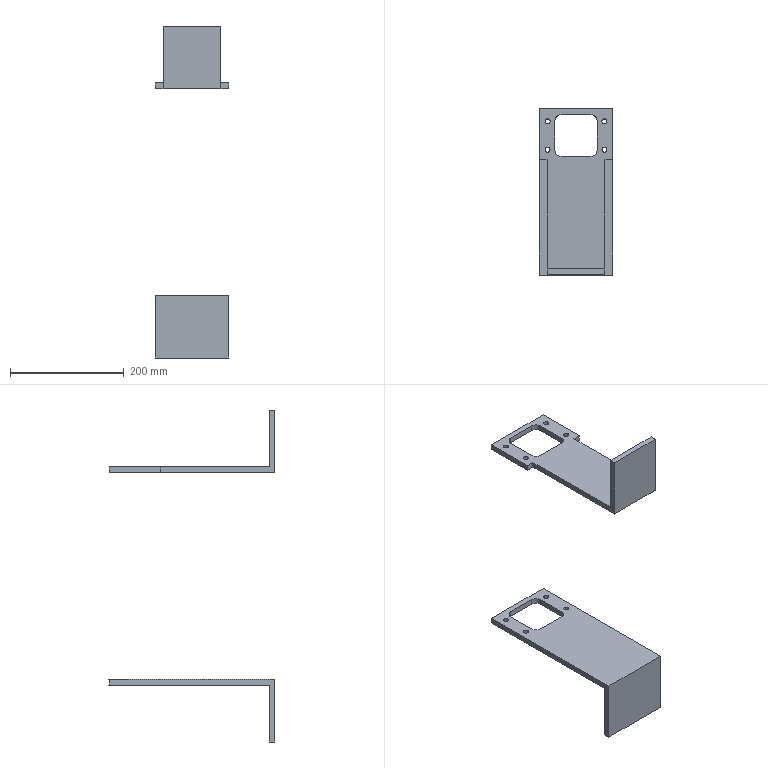Part | NX | 2 solids | 44 faces | box 129 x 292 x 584 mm | volume 817102 mm3 | plane 28 | cylinder 16 | commonest cylinder face diameters 9 x8 21.378 x8
STEP:
#1=CARTESIAN_POINT('',(4645.75,76.144,-128.));
#2=VERTEX_POINT('',#1);
#3=CARTESIAN_POINT('',(4659.262,76.144,-128.));
#4=VERTEX_POINT('',#3);
#5=CARTESIAN_POINT('',(4098.348,76.144,-128.));
#6=DIRECTION('',(1.,0.,0.));
#7=VECTOR('',#6,1.);
#8=LINE('',#5,#7);
#9=EDGE_CURVE('',#2,#4,#8,.T.);
#10=ORIENTED_EDGE('',*,*,#9,.F.);
#11=CARTESIAN_POINT('',(4645.75,76.144,-138.));
#12=VERTEX_POINT('',#11);
#13=CARTESIAN_POINT('',(4645.75,76.144,-128.));
#14=DIRECTION('',(0.,0.,1.));
#15=VECTOR('',#14,1.);
#16=LINE('',#13,#15);
#17=EDGE_CURVE('',#12,#2,#16,.T.);
#18=ORIENTED_EDGE('',*,*,#17,.F.);
#19=CARTESIAN_POINT('',(4659.262,76.144,-138.));
#20=VERTEX_POINT('',#19);
#21=CARTESIAN_POINT('',(4098.348,76.144,-138.));
#22=DIRECTION('',(-1.,0.,0.));
#23=VECTOR('',#22,1.);
#24=LINE('',#21,#23);
#25=EDGE_CURVE('',#20,#12,#24,.T.);
#26=ORIENTED_EDGE('',*,*,#25,.F.);
#27=CARTESIAN_POINT('',(4659.262,76.144,-150.));
#28=DIRECTION('',(0.,0.,1.));
#29=VECTOR('',#28,1.);
#30=LINE('',#27,#29);
#31=EDGE_CURVE('',#20,#4,#30,.T.);
#32=ORIENTED_EDGE('',*,*,#31,.T.);
#33=EDGE_LOOP('',(#10,#18,#26,#32));
#34=FACE_OUTER_BOUND('',#33,.T.);
#35=CARTESIAN_POINT('',(9954.033,76.144,0.));
#36=DIRECTION('',(0.,1.,0.));
#37=DIRECTION('',(0.,0.,1.));
#38=AXIS2_PLACEMENT_3D('',#35,#36,#37);
#39=PLANE('',#38);
#40=ADVANCED_FACE('',(#34),#39,.F.);
#41=CARTESIAN_POINT('',(4659.262,-125.856,-138.));
#42=VERTEX_POINT('',#41);
#43=CARTESIAN_POINT('',(4659.262,-499.191,-138.));
#44=DIRECTION('',(0.,1.,0.));
#45=VECTOR('',#44,1.);
#46=LINE('',#43,#45);
#47=EDGE_CURVE('',#42,#20,#46,.T.);
#48=ORIENTED_EDGE('',*,*,#47,.F.);
#49=CARTESIAN_POINT('',(4659.262,-125.856,-28.));
#50=VERTEX_POINT('',#49);
#51=CARTESIAN_POINT('',(4659.262,-125.856,-150.));
#52=DIRECTION('',(0.,0.,-1.));
#53=VECTOR('',#52,1.);
#54=LINE('',#51,#53);
#55=EDGE_CURVE('',#50,#42,#54,.T.);
#56=ORIENTED_EDGE('',*,*,#55,.F.);
#57=CARTESIAN_POINT('',(4659.262,-115.856,-28.));
#58=VERTEX_POINT('',#57);
#59=CARTESIAN_POINT('',(4659.262,-125.856,-28.));
#60=DIRECTION('',(0.,-1.,0.));
#61=VECTOR('',#60,1.);
#62=LINE('',#59,#61);
#63=EDGE_CURVE('',#58,#50,#62,.T.);
#64=ORIENTED_EDGE('',*,*,#63,.F.);
#65=CARTESIAN_POINT('',(4659.262,-115.856,-128.));
#66=VERTEX_POINT('',#65);
#67=CARTESIAN_POINT('',(4659.262,-115.856,-128.));
#68=DIRECTION('',(0.,0.,1.));
#69=VECTOR('',#68,1.);
#70=LINE('',#67,#69);
#71=EDGE_CURVE('',#66,#58,#70,.T.);
#72=ORIENTED_EDGE('',*,*,#71,.F.);
#73=CARTESIAN_POINT('',(4659.262,-499.191,-128.));
#74=DIRECTION('',(0.,-1.,0.));
#75=VECTOR('',#74,1.);
#76=LINE('',#73,#75);
#77=EDGE_CURVE('',#4,#66,#76,.T.);
#78=ORIENTED_EDGE('',*,*,#77,.F.);
#79=ORIENTED_EDGE('',*,*,#31,.F.);
#80=EDGE_LOOP('',(#48,#56,#64,#72,#78,#79));
#81=FACE_OUTER_BOUND('',#80,.T.);
#82=CARTESIAN_POINT('',(4659.262,-45.856,-150.));
#83=DIRECTION('',(-1.,0.,0.));
#84=DIRECTION('',(0.,0.,-1.));
#85=AXIS2_PLACEMENT_3D('',#82,#83,#84);
#86=PLANE('',#85);
#87=ADVANCED_FACE('',(#81),#86,.T.);
#88=CARTESIAN_POINT('',(4774.75,76.144,-128.));
#89=VERTEX_POINT('',#88);
#90=CARTESIAN_POINT('',(4761.238,76.144,-128.));
#91=VERTEX_POINT('',#90);
#92=CARTESIAN_POINT('',(5322.152,76.144,-128.));
#93=DIRECTION('',(-1.,0.,0.));
#94=VECTOR('',#93,1.);
#95=LINE('',#92,#94);
#96=EDGE_CURVE('',#89,#91,#95,.T.);
#97=ORIENTED_EDGE('',*,*,#96,.T.);
#98=CARTESIAN_POINT('',(4761.238,76.144,-138.));
#99=VERTEX_POINT('',#98);
#100=CARTESIAN_POINT('',(4761.238,76.144,-150.));
#101=DIRECTION('',(0.,0.,-1.));
#102=VECTOR('',#101,1.);
#103=LINE('',#100,#102);
#104=EDGE_CURVE('',#91,#99,#103,.T.);
#105=ORIENTED_EDGE('',*,*,#104,.T.);
#106=CARTESIAN_POINT('',(4774.75,76.144,-138.));
#107=VERTEX_POINT('',#106);
#108=CARTESIAN_POINT('',(5322.152,76.144,-138.));
#109=DIRECTION('',(-1.,0.,0.));
#110=VECTOR('',#109,1.);
#111=LINE('',#108,#110);
#112=EDGE_CURVE('',#107,#99,#111,.T.);
#113=ORIENTED_EDGE('',*,*,#112,.F.);
#114=CARTESIAN_POINT('',(4774.75,76.144,-128.));
#115=DIRECTION('',(0.,0.,-1.));
#116=VECTOR('',#115,1.);
#117=LINE('',#114,#116);
#118=EDGE_CURVE('',#89,#107,#117,.T.);
#119=ORIENTED_EDGE('',*,*,#118,.F.);
#120=EDGE_LOOP('',(#97,#105,#113,#119));
#121=FACE_OUTER_BOUND('',#120,.T.);
#122=CARTESIAN_POINT('',(-533.533,76.144,0.));
#123=DIRECTION('',(0.,1.,0.));
#124=DIRECTION('',(0.,0.,1.));
#125=AXIS2_PLACEMENT_3D('',#122,#123,#124);
#126=PLANE('',#125);
#127=ADVANCED_FACE('',(#121),#126,.F.);
#128=CARTESIAN_POINT('',(4774.75,166.144,-128.));
#129=VERTEX_POINT('',#128);
#130=CARTESIAN_POINT('',(4774.75,-125.856,-128.));
#131=DIRECTION('',(0.,1.,0.));
#132=VECTOR('',#131,1.);
#133=LINE('',#130,#132);
#134=EDGE_CURVE('',#89,#129,#133,.T.);
#135=ORIENTED_EDGE('',*,*,#134,.F.);
#136=ORIENTED_EDGE('',*,*,#118,.T.);
#137=CARTESIAN_POINT('',(4774.75,166.144,-138.));
#138=VERTEX_POINT('',#137);
#139=CARTESIAN_POINT('',(4774.75,-125.856,-138.));
#140=DIRECTION('',(0.,1.,0.));
#141=VECTOR('',#140,1.);
#142=LINE('',#139,#141);
#143=EDGE_CURVE('',#107,#138,#142,.T.);
#144=ORIENTED_EDGE('',*,*,#143,.T.);
#145=CARTESIAN_POINT('',(4774.75,166.144,-128.));
#146=DIRECTION('',(0.,0.,-1.));
#147=VECTOR('',#146,1.);
#148=LINE('',#145,#147);
#149=EDGE_CURVE('',#129,#138,#148,.T.);
#150=ORIENTED_EDGE('',*,*,#149,.F.);
#151=EDGE_LOOP('',(#135,#136,#144,#150));
#152=FACE_OUTER_BOUND('',#151,.T.);
#153=CARTESIAN_POINT('',(4774.75,-125.856,-128.));
#154=DIRECTION('',(-1.,0.,0.));
#155=DIRECTION('',(0.,0.,-1.));
#156=AXIS2_PLACEMENT_3D('',#153,#154,#155);
#157=PLANE('',#156);
#158=ADVANCED_FACE('',(#152),#157,.F.);
#159=CARTESIAN_POINT('',(4660.25,139.644,-138.));
#160=VERTEX_POINT('',#159);
#161=CARTESIAN_POINT('',(4660.25,144.144,-138.));
#162=DIRECTION('',(0.,0.,1.));
#163=DIRECTION('',(0.,-1.,0.));
#164=AXIS2_PLACEMENT_3D('',#161,#162,#163);
#165=CIRCLE('',#164,4.5);
#166=EDGE_CURVE('',#160,#160,#165,.T.);
#167=ORIENTED_EDGE('',*,*,#166,.F.);
#168=EDGE_LOOP('',(#167));
#169=FACE_BOUND('',#168,.T.);
#170=CARTESIAN_POINT('',(4660.25,139.644,-128.));
#171=VERTEX_POINT('',#170);
#172=CARTESIAN_POINT('',(4660.25,144.144,-128.));
#173=DIRECTION('',(0.,0.,1.));
#174=DIRECTION('',(0.,-1.,0.));
#175=AXIS2_PLACEMENT_3D('',#172,#173,#174);
#176=CIRCLE('',#175,4.5);
#177=EDGE_CURVE('',#171,#171,#176,.T.);
#178=ORIENTED_EDGE('',*,*,#177,.T.);
#179=EDGE_LOOP('',(#178));
#180=FACE_BOUND('',#179,.T.);
#181=CARTESIAN_POINT('',(4660.25,144.144,-128.));
#182=DIRECTION('',(0.,0.,-1.));
#183=DIRECTION('',(1.,0.,0.));
#184=AXIS2_PLACEMENT_3D('',#181,#182,#183);
#185=CYLINDRICAL_SURFACE('',#184,4.5);
#186=ADVANCED_FACE('',(#169,#180),#185,.F.);
#187=CARTESIAN_POINT('',(4736.561,156.144,-138.));
#188=VERTEX_POINT('',#187);
#189=CARTESIAN_POINT('',(4747.25,145.455,-138.));
#190=VERTEX_POINT('',#189);
#191=CARTESIAN_POINT('',(4736.561,145.455,-138.));
#192=DIRECTION('',(0.,0.,-1.));
#193=DIRECTION('',(0.,1.,0.));
#194=AXIS2_PLACEMENT_3D('',#191,#192,#193);
#195=CIRCLE('',#194,10.689);
#196=EDGE_CURVE('',#188,#190,#195,.T.);
#197=ORIENTED_EDGE('',*,*,#196,.T.);
#198=CARTESIAN_POINT('',(4747.25,145.455,-128.));
#199=VERTEX_POINT('',#198);
#200=CARTESIAN_POINT('',(4747.25,145.455,-128.));
#201=DIRECTION('',(0.,0.,1.));
#202=VECTOR('',#201,1.);
#203=LINE('',#200,#202);
#204=EDGE_CURVE('',#190,#199,#203,.T.);
#205=ORIENTED_EDGE('',*,*,#204,.T.);
#206=CARTESIAN_POINT('',(4736.561,156.144,-128.));
#207=VERTEX_POINT('',#206);
#208=CARTESIAN_POINT('',(4736.561,145.455,-128.));
#209=DIRECTION('',(0.,0.,-1.));
#210=DIRECTION('',(0.,1.,0.));
#211=AXIS2_PLACEMENT_3D('',#208,#209,#210);
#212=CIRCLE('',#211,10.689);
#213=EDGE_CURVE('',#207,#199,#212,.T.);
#214=ORIENTED_EDGE('',*,*,#213,.F.);
#215=CARTESIAN_POINT('',(4736.561,156.144,-128.));
#216=DIRECTION('',(0.,0.,1.));
#217=VECTOR('',#216,1.);
#218=LINE('',#215,#217);
#219=EDGE_CURVE('',#188,#207,#218,.T.);
#220=ORIENTED_EDGE('',*,*,#219,.F.);
#221=EDGE_LOOP('',(#197,#205,#214,#220));
#222=FACE_OUTER_BOUND('',#221,.T.);
#223=CARTESIAN_POINT('',(4736.561,145.455,-128.));
#224=DIRECTION('',(0.,0.,-1.));
#225=DIRECTION('',(1.,0.,0.));
#226=AXIS2_PLACEMENT_3D('',#223,#224,#225);
#227=CYLINDRICAL_SURFACE('',#226,10.689);
#228=ADVANCED_FACE('',(#222),#227,.F.);
#229=CARTESIAN_POINT('',(4747.25,92.834,-138.));
#230=VERTEX_POINT('',#229);
#231=CARTESIAN_POINT('',(4747.25,145.455,-138.));
#232=DIRECTION('',(0.,-1.,0.));
#233=VECTOR('',#232,1.);
#234=LINE('',#231,#233);
#235=EDGE_CURVE('',#190,#230,#234,.T.);
#236=ORIENTED_EDGE('',*,*,#235,.T.);
#237=CARTESIAN_POINT('',(4747.25,92.834,-128.));
#238=VERTEX_POINT('',#237);
#239=CARTESIAN_POINT('',(4747.25,92.834,-128.));
#240=DIRECTION('',(0.,0.,1.));
#241=VECTOR('',#240,1.);
#242=LINE('',#239,#241);
#243=EDGE_CURVE('',#230,#238,#242,.T.);
#244=ORIENTED_EDGE('',*,*,#243,.T.);
#245=CARTESIAN_POINT('',(4747.25,145.455,-128.));
#246=DIRECTION('',(0.,-1.,0.));
#247=VECTOR('',#246,1.);
#248=LINE('',#245,#247);
#249=EDGE_CURVE('',#199,#238,#248,.T.);
#250=ORIENTED_EDGE('',*,*,#249,.F.);
#251=ORIENTED_EDGE('',*,*,#204,.F.);
#252=EDGE_LOOP('',(#236,#244,#250,#251));
#253=FACE_OUTER_BOUND('',#252,.T.);
#254=CARTESIAN_POINT('',(4747.25,145.455,-128.));
#255=DIRECTION('',(1.,0.,0.));
#256=DIRECTION('',(0.,0.,1.));
#257=AXIS2_PLACEMENT_3D('',#254,#255,#256);
#258=PLANE('',#257);
#259=ADVANCED_FACE('',(#253),#258,.F.);
#260=CARTESIAN_POINT('',(4736.561,82.144,-138.));
#261=VERTEX_POINT('',#260);
#262=CARTESIAN_POINT('',(4736.561,92.834,-138.));
#263=DIRECTION('',(0.,0.,-1.));
#264=DIRECTION('',(0.,1.,0.));
#265=AXIS2_PLACEMENT_3D('',#262,#263,#264);
#266=CIRCLE('',#265,10.689);
#267=EDGE_CURVE('',#230,#261,#266,.T.);
#268=ORIENTED_EDGE('',*,*,#267,.T.);
#269=CARTESIAN_POINT('',(4736.561,82.144,-128.));
#270=VERTEX_POINT('',#269);
#271=CARTESIAN_POINT('',(4736.561,82.144,-128.));
#272=DIRECTION('',(0.,0.,1.));
#273=VECTOR('',#272,1.);
#274=LINE('',#271,#273);
#275=EDGE_CURVE('',#261,#270,#274,.T.);
#276=ORIENTED_EDGE('',*,*,#275,.T.);
#277=CARTESIAN_POINT('',(4736.561,92.834,-128.));
#278=DIRECTION('',(0.,0.,-1.));
#279=DIRECTION('',(0.,1.,0.));
#280=AXIS2_PLACEMENT_3D('',#277,#278,#279);
#281=CIRCLE('',#280,10.689);
#282=EDGE_CURVE('',#238,#270,#281,.T.);
#283=ORIENTED_EDGE('',*,*,#282,.F.);
#284=ORIENTED_EDGE('',*,*,#243,.F.);
#285=EDGE_LOOP('',(#268,#276,#283,#284));
#286=FACE_OUTER_BOUND('',#285,.T.);
#287=CARTESIAN_POINT('',(4736.561,92.834,-128.));
#288=DIRECTION('',(0.,0.,-1.));
#289=DIRECTION('',(1.,0.,0.));
#290=AXIS2_PLACEMENT_3D('',#287,#288,#289);
#291=CYLINDRICAL_SURFACE('',#290,10.689);
#292=ADVANCED_FACE('',(#286),#291,.F.);
#293=CARTESIAN_POINT('',(4683.939,82.144,-138.));
#294=VERTEX_POINT('',#293);
#295=CARTESIAN_POINT('',(4736.561,82.144,-138.));
#296=DIRECTION('',(-1.,0.,0.));
#297=VECTOR('',#296,1.);
#298=LINE('',#295,#297);
#299=EDGE_CURVE('',#261,#294,#298,.T.);
#300=ORIENTED_EDGE('',*,*,#299,.T.);
#301=CARTESIAN_POINT('',(4683.939,82.144,-128.));
#302=VERTEX_POINT('',#301);
#303=CARTESIAN_POINT('',(4683.939,82.144,-128.));
#304=DIRECTION('',(0.,0.,1.));
#305=VECTOR('',#304,1.);
#306=LINE('',#303,#305);
#307=EDGE_CURVE('',#294,#302,#306,.T.);
#308=ORIENTED_EDGE('',*,*,#307,.T.);
#309=CARTESIAN_POINT('',(4736.561,82.144,-128.));
#310=DIRECTION('',(-1.,0.,0.));
#311=VECTOR('',#310,1.);
#312=LINE('',#309,#311);
#313=EDGE_CURVE('',#270,#302,#312,.T.);
#314=ORIENTED_EDGE('',*,*,#313,.F.);
#315=ORIENTED_EDGE('',*,*,#275,.F.);
#316=EDGE_LOOP('',(#300,#308,#314,#315));
#317=FACE_OUTER_BOUND('',#316,.T.);
#318=CARTESIAN_POINT('',(4736.561,82.144,-128.));
#319=DIRECTION('',(0.,-1.,0.));
#320=DIRECTION('',(1.,0.,0.));
#321=AXIS2_PLACEMENT_3D('',#318,#319,#320);
#322=PLANE('',#321);
#323=ADVANCED_FACE('',(#317),#322,.F.);
#324=CARTESIAN_POINT('',(4673.25,92.834,-138.));
#325=VERTEX_POINT('',#324);
#326=CARTESIAN_POINT('',(4683.939,92.834,-138.));
#327=DIRECTION('',(0.,0.,-1.));
#328=DIRECTION('',(0.,1.,0.));
#329=AXIS2_PLACEMENT_3D('',#326,#327,#328);
#330=CIRCLE('',#329,10.689);
#331=EDGE_CURVE('',#294,#325,#330,.T.);
#332=ORIENTED_EDGE('',*,*,#331,.T.);
#333=CARTESIAN_POINT('',(4673.25,92.834,-128.));
#334=VERTEX_POINT('',#333);
#335=CARTESIAN_POINT('',(4673.25,92.834,-128.));
#336=DIRECTION('',(0.,0.,1.));
#337=VECTOR('',#336,1.);
#338=LINE('',#335,#337);
#339=EDGE_CURVE('',#325,#334,#338,.T.);
#340=ORIENTED_EDGE('',*,*,#339,.T.);
#341=CARTESIAN_POINT('',(4683.939,92.834,-128.));
#342=DIRECTION('',(0.,0.,-1.));
#343=DIRECTION('',(0.,1.,0.));
#344=AXIS2_PLACEMENT_3D('',#341,#342,#343);
#345=CIRCLE('',#344,10.689);
#346=EDGE_CURVE('',#302,#334,#345,.T.);
#347=ORIENTED_EDGE('',*,*,#346,.F.);
#348=ORIENTED_EDGE('',*,*,#307,.F.);
#349=EDGE_LOOP('',(#332,#340,#347,#348));
#350=FACE_OUTER_BOUND('',#349,.T.);
#351=CARTESIAN_POINT('',(4683.939,92.834,-128.));
#352=DIRECTION('',(0.,0.,-1.));
#353=DIRECTION('',(1.,0.,0.));
#354=AXIS2_PLACEMENT_3D('',#351,#352,#353);
#355=CYLINDRICAL_SURFACE('',#354,10.689);
#356=ADVANCED_FACE('',(#350),#355,.F.);
#357=CARTESIAN_POINT('',(4673.25,145.455,-138.));
#358=VERTEX_POINT('',#357);
#359=CARTESIAN_POINT('',(4673.25,92.834,-138.));
#360=DIRECTION('',(0.,1.,0.));
#361=VECTOR('',#360,1.);
#362=LINE('',#359,#361);
#363=EDGE_CURVE('',#325,#358,#362,.T.);
#364=ORIENTED_EDGE('',*,*,#363,.T.);
#365=CARTESIAN_POINT('',(4673.25,145.455,-128.));
#366=VERTEX_POINT('',#365);
#367=CARTESIAN_POINT('',(4673.25,145.455,-128.));
#368=DIRECTION('',(0.,0.,1.));
#369=VECTOR('',#368,1.);
#370=LINE('',#367,#369);
#371=EDGE_CURVE('',#358,#366,#370,.T.);
#372=ORIENTED_EDGE('',*,*,#371,.T.);
#373=CARTESIAN_POINT('',(4673.25,92.834,-128.));
#374=DIRECTION('',(0.,1.,0.));
#375=VECTOR('',#374,1.);
#376=LINE('',#373,#375);
#377=EDGE_CURVE('',#334,#366,#376,.T.);
#378=ORIENTED_EDGE('',*,*,#377,.F.);
#379=ORIENTED_EDGE('',*,*,#339,.F.);
#380=EDGE_LOOP('',(#364,#372,#378,#379));
#381=FACE_OUTER_BOUND('',#380,.T.);
#382=CARTESIAN_POINT('',(4673.25,92.834,-128.));
#383=DIRECTION('',(-1.,0.,0.));
#384=DIRECTION('',(0.,0.,-1.));
#385=AXIS2_PLACEMENT_3D('',#382,#383,#384);
#386=PLANE('',#385);
#387=ADVANCED_FACE('',(#381),#386,.F.);
#388=CARTESIAN_POINT('',(4683.939,156.144,-138.));
#389=VERTEX_POINT('',#388);
#390=CARTESIAN_POINT('',(4683.939,145.455,-138.));
#391=DIRECTION('',(0.,0.,-1.));
#392=DIRECTION('',(0.,1.,0.));
#393=AXIS2_PLACEMENT_3D('',#390,#391,#392);
#394=CIRCLE('',#393,10.689);
#395=EDGE_CURVE('',#358,#389,#394,.T.);
#396=ORIENTED_EDGE('',*,*,#395,.T.);
#397=CARTESIAN_POINT('',(4683.939,156.144,-128.));
#398=VERTEX_POINT('',#397);
#399=CARTESIAN_POINT('',(4683.939,156.144,-128.));
#400=DIRECTION('',(0.,0.,1.));
#401=VECTOR('',#400,1.);
#402=LINE('',#399,#401);
#403=EDGE_CURVE('',#389,#398,#402,.T.);
#404=ORIENTED_EDGE('',*,*,#403,.T.);
#405=CARTESIAN_POINT('',(4683.939,145.455,-128.));
#406=DIRECTION('',(0.,0.,-1.));
#407=DIRECTION('',(0.,1.,0.));
#408=AXIS2_PLACEMENT_3D('',#405,#406,#407);
#409=CIRCLE('',#408,10.689);
#410=EDGE_CURVE('',#366,#398,#409,.T.);
#411=ORIENTED_EDGE('',*,*,#410,.F.);
#412=ORIENTED_EDGE('',*,*,#371,.F.);
#413=EDGE_LOOP('',(#396,#404,#411,#412));
#414=FACE_OUTER_BOUND('',#413,.T.);
#415=CARTESIAN_POINT('',(4683.939,145.455,-128.));
#416=DIRECTION('',(0.,0.,-1.));
#417=DIRECTION('',(1.,0.,0.));
#418=AXIS2_PLACEMENT_3D('',#415,#416,#417);
#419=CYLINDRICAL_SURFACE('',#418,10.689);
#420=ADVANCED_FACE('',(#414),#419,.F.);
#421=CARTESIAN_POINT('',(4683.939,156.144,-138.));
#422=DIRECTION('',(1.,0.,0.));
#423=VECTOR('',#422,1.);
#424=LINE('',#421,#423);
#425=EDGE_CURVE('',#389,#188,#424,.T.);
#426=ORIENTED_EDGE('',*,*,#425,.T.);
#427=ORIENTED_EDGE('',*,*,#219,.T.);
#428=CARTESIAN_POINT('',(4683.939,156.144,-128.));
#429=DIRECTION('',(1.,0.,0.));
#430=VECTOR('',#429,1.);
#431=LINE('',#428,#430);
#432=EDGE_CURVE('',#398,#207,#431,.T.);
#433=ORIENTED_EDGE('',*,*,#432,.F.);
#434=ORIENTED_EDGE('',*,*,#403,.F.);
#435=EDGE_LOOP('',(#426,#427,#433,#434));
#436=FACE_OUTER_BOUND('',#435,.T.);
#437=CARTESIAN_POINT('',(4683.939,156.144,-128.));
#438=DIRECTION('',(0.,1.,0.));
#439=DIRECTION('',(-1.,0.,0.));
#440=AXIS2_PLACEMENT_3D('',#437,#438,#439);
#441=PLANE('',#440);
#442=ADVANCED_FACE('',(#436),#441,.F.);
#443=CARTESIAN_POINT('',(4760.25,89.644,-138.));
#444=VERTEX_POINT('',#443);
#445=CARTESIAN_POINT('',(4760.25,94.144,-138.));
#446=DIRECTION('',(0.,0.,-1.));
#447=DIRECTION('',(0.,-1.,0.));
#448=AXIS2_PLACEMENT_3D('',#445,#446,#447);
#449=CIRCLE('',#448,4.5);
#450=EDGE_CURVE('',#444,#444,#449,.T.);
#451=ORIENTED_EDGE('',*,*,#450,.T.);
#452=EDGE_LOOP('',(#451));
#453=FACE_BOUND('',#452,.T.);
#454=CARTESIAN_POINT('',(4760.25,89.644,-128.));
#455=VERTEX_POINT('',#454);
#456=CARTESIAN_POINT('',(4760.25,94.144,-128.));
#457=DIRECTION('',(0.,0.,-1.));
#458=DIRECTION('',(0.,-1.,0.));
#459=AXIS2_PLACEMENT_3D('',#456,#457,#458);
#460=CIRCLE('',#459,4.5);
#461=EDGE_CURVE('',#455,#455,#460,.T.);
#462=ORIENTED_EDGE('',*,*,#461,.F.);
#463=EDGE_LOOP('',(#462));
#464=FACE_BOUND('',#463,.T.);
#465=CARTESIAN_POINT('',(4760.25,94.144,-128.));
#466=DIRECTION('',(0.,0.,-1.));
#467=DIRECTION('',(1.,0.,0.));
#468=AXIS2_PLACEMENT_3D('',#465,#466,#467);
#469=CYLINDRICAL_SURFACE('',#468,4.5);
#470=ADVANCED_FACE('',(#453,#464),#469,.F.);
#471=CARTESIAN_POINT('',(4760.25,139.644,-138.));
#472=VERTEX_POINT('',#471);
#473=CARTESIAN_POINT('',(4760.25,144.144,-138.));
#474=DIRECTION('',(0.,0.,-1.));
#475=DIRECTION('',(0.,-1.,0.));
#476=AXIS2_PLACEMENT_3D('',#473,#474,#475);
#477=CIRCLE('',#476,4.5);
#478=EDGE_CURVE('',#472,#472,#477,.T.);
#479=ORIENTED_EDGE('',*,*,#478,.T.);
#480=EDGE_LOOP('',(#479));
#481=FACE_BOUND('',#480,.T.);
#482=CARTESIAN_POINT('',(4760.25,139.644,-128.));
#483=VERTEX_POINT('',#482);
#484=CARTESIAN_POINT('',(4760.25,144.144,-128.));
#485=DIRECTION('',(0.,0.,-1.));
#486=DIRECTION('',(0.,-1.,0.));
#487=AXIS2_PLACEMENT_3D('',#484,#485,#486);
#488=CIRCLE('',#487,4.5);
#489=EDGE_CURVE('',#483,#483,#488,.T.);
#490=ORIENTED_EDGE('',*,*,#489,.F.);
#491=EDGE_LOOP('',(#490));
#492=FACE_BOUND('',#491,.T.);
#493=CARTESIAN_POINT('',(4760.25,144.144,-128.));
#494=DIRECTION('',(0.,0.,-1.));
#495=DIRECTION('',(1.,0.,0.));
#496=AXIS2_PLACEMENT_3D('',#493,#494,#495);
#497=CYLINDRICAL_SURFACE('',#496,4.5);
#498=ADVANCED_FACE('',(#481,#492),#497,.F.);
#499=CARTESIAN_POINT('',(4660.25,89.644,-138.));
#500=VERTEX_POINT('',#499);
#501=CARTESIAN_POINT('',(4660.25,94.144,-138.));
#502=DIRECTION('',(0.,0.,-1.));
#503=DIRECTION('',(0.,-1.,0.));
#504=AXIS2_PLACEMENT_3D('',#501,#502,#503);
#505=CIRCLE('',#504,4.5);
#506=EDGE_CURVE('',#500,#500,#505,.T.);
#507=ORIENTED_EDGE('',*,*,#506,.T.);
#508=EDGE_LOOP('',(#507));
#509=FACE_BOUND('',#508,.T.);
#510=CARTESIAN_POINT('',(4660.25,89.644,-128.));
#511=VERTEX_POINT('',#510);
#512=CARTESIAN_POINT('',(4660.25,94.144,-128.));
#513=DIRECTION('',(0.,0.,-1.));
#514=DIRECTION('',(0.,-1.,0.));
#515=AXIS2_PLACEMENT_3D('',#512,#513,#514);
#516=CIRCLE('',#515,4.5);
#517=EDGE_CURVE('',#511,#511,#516,.T.);
#518=ORIENTED_EDGE('',*,*,#517,.F.);
#519=EDGE_LOOP('',(#518));
#520=FACE_BOUND('',#519,.T.);
#521=CARTESIAN_POINT('',(4660.25,94.144,-128.));
#522=DIRECTION('',(0.,0.,-1.));
#523=DIRECTION('',(1.,0.,0.));
#524=AXIS2_PLACEMENT_3D('',#521,#522,#523);
#525=CYLINDRICAL_SURFACE('',#524,4.5);
#526=ADVANCED_FACE('',(#509,#520),#525,.F.);
#527=CARTESIAN_POINT('',(4645.75,166.144,-138.));
#528=VERTEX_POINT('',#527);
#529=CARTESIAN_POINT('',(4774.75,166.144,-138.));
#530=DIRECTION('',(-1.,0.,0.));
#531=VECTOR('',#530,1.);
#532=LINE('',#529,#531);
#533=EDGE_CURVE('',#138,#528,#532,.T.);
#534=ORIENTED_EDGE('',*,*,#533,.T.);
#535=CARTESIAN_POINT('',(4645.75,166.144,-128.));
#536=VERTEX_POINT('',#535);
#537=CARTESIAN_POINT('',(4645.75,166.144,-128.));
#538=DIRECTION('',(0.,0.,-1.));
#539=VECTOR('',#538,1.);
#540=LINE('',#537,#539);
#541=EDGE_CURVE('',#536,#528,#540,.T.);
#542=ORIENTED_EDGE('',*,*,#541,.F.);
#543=CARTESIAN_POINT('',(4774.75,166.144,-128.));
#544=DIRECTION('',(-1.,0.,0.));
#545=VECTOR('',#544,1.);
#546=LINE('',#543,#545);
#547=EDGE_CURVE('',#129,#536,#546,.T.);
#548=ORIENTED_EDGE('',*,*,#547,.F.);
#549=ORIENTED_EDGE('',*,*,#149,.T.);
#550=EDGE_LOOP('',(#534,#542,#548,#549));
#551=FACE_OUTER_BOUND('',#550,.T.);
#552=CARTESIAN_POINT('',(4774.75,166.144,-128.));
#553=DIRECTION('',(0.,-1.,0.));
#554=DIRECTION('',(0.,0.,-1.));
#555=AXIS2_PLACEMENT_3D('',#552,#553,#554);
#556=PLANE('',#555);
#557=ADVANCED_FACE('',(#551),#556,.F.);
#558=ORIENTED_EDGE('',*,*,#489,.T.);
#559=EDGE_LOOP('',(#558));
#560=FACE_BOUND('',#559,.T.);
#561=ORIENTED_EDGE('',*,*,#410,.T.);
#562=ORIENTED_EDGE('',*,*,#432,.T.);
#563=ORIENTED_EDGE('',*,*,#213,.T.);
#564=ORIENTED_EDGE('',*,*,#249,.T.);
#565=ORIENTED_EDGE('',*,*,#282,.T.);
#566=ORIENTED_EDGE('',*,*,#313,.T.);
#567=ORIENTED_EDGE('',*,*,#346,.T.);
#568=ORIENTED_EDGE('',*,*,#377,.T.);
#569=EDGE_LOOP('',(#561,#562,#563,#564,#565,#566,#567,#568));
#570=FACE_BOUND('',#569,.T.);
#571=ORIENTED_EDGE('',*,*,#177,.F.);
#572=EDGE_LOOP('',(#571));
#573=FACE_BOUND('',#572,.T.);
#574=ORIENTED_EDGE('',*,*,#461,.T.);
#575=EDGE_LOOP('',(#574));
#576=FACE_BOUND('',#575,.T.);
#577=ORIENTED_EDGE('',*,*,#517,.T.);
#578=EDGE_LOOP('',(#577));
#579=FACE_BOUND('',#578,.T.);
#580=CARTESIAN_POINT('',(4645.75,156.144,-128.));
#581=DIRECTION('',(0.,-1.,0.));
#582=VECTOR('',#581,1.);
#583=LINE('',#580,#582);
#584=EDGE_CURVE('',#536,#2,#583,.T.);
#585=ORIENTED_EDGE('',*,*,#584,.T.);
#586=ORIENTED_EDGE('',*,*,#9,.T.);
#587=ORIENTED_EDGE('',*,*,#77,.T.);
#588=CARTESIAN_POINT('',(4761.238,-115.856,-128.));
#589=VERTEX_POINT('',#588);
#590=CARTESIAN_POINT('',(4645.75,-115.856,-128.));
#591=DIRECTION('',(1.,0.,0.));
#592=VECTOR('',#591,1.);
#593=LINE('',#590,#592);
#594=EDGE_CURVE('',#66,#589,#593,.T.);
#595=ORIENTED_EDGE('',*,*,#594,.T.);
#596=CARTESIAN_POINT('',(4761.238,-499.191,-128.));
#597=DIRECTION('',(0.,1.,0.));
#598=VECTOR('',#597,1.);
#599=LINE('',#596,#598);
#600=EDGE_CURVE('',#589,#91,#599,.T.);
#601=ORIENTED_EDGE('',*,*,#600,.T.);
#602=ORIENTED_EDGE('',*,*,#96,.F.);
#603=ORIENTED_EDGE('',*,*,#134,.T.);
#604=ORIENTED_EDGE('',*,*,#547,.T.);
#605=EDGE_LOOP('',(#585,#586,#587,#595,#601,#602,#603,#604));
#606=FACE_BOUND('',#605,.T.);
#607=CARTESIAN_POINT('',(5322.152,-499.191,-128.));
#608=DIRECTION('',(0.,0.,1.));
#609=DIRECTION('',(-1.,0.,0.));
#610=AXIS2_PLACEMENT_3D('',#607,#608,#609);
#611=PLANE('',#610);
#612=ADVANCED_FACE('',(#560,#570,#573,#576,#579,#606),#611,.T.);
#613=CARTESIAN_POINT('',(4761.238,-125.856,-138.));
#614=VERTEX_POINT('',#613);
#615=CARTESIAN_POINT('',(4761.238,-499.191,-138.));
#616=DIRECTION('',(0.,1.,0.));
#617=VECTOR('',#616,1.);
#618=LINE('',#615,#617);
#619=EDGE_CURVE('',#614,#99,#618,.T.);
#620=ORIENTED_EDGE('',*,*,#619,.T.);
#621=ORIENTED_EDGE('',*,*,#104,.F.);
#622=ORIENTED_EDGE('',*,*,#600,.F.);
#623=CARTESIAN_POINT('',(4761.238,-115.856,-28.));
#624=VERTEX_POINT('',#623);
#625=CARTESIAN_POINT('',(4761.238,-115.856,-128.));
#626=DIRECTION('',(0.,0.,1.));
#627=VECTOR('',#626,1.);
#628=LINE('',#625,#627);
#629=EDGE_CURVE('',#589,#624,#628,.T.);
#630=ORIENTED_EDGE('',*,*,#629,.T.);
#631=CARTESIAN_POINT('',(4761.238,-125.856,-28.));
#632=VERTEX_POINT('',#631);
#633=CARTESIAN_POINT('',(4761.238,-125.856,-28.));
#634=DIRECTION('',(0.,-1.,0.));
#635=VECTOR('',#634,1.);
#636=LINE('',#633,#635);
#637=EDGE_CURVE('',#624,#632,#636,.T.);
#638=ORIENTED_EDGE('',*,*,#637,.T.);
#639=CARTESIAN_POINT('',(4761.238,-125.856,-150.));
#640=DIRECTION('',(0.,0.,1.));
#641=VECTOR('',#640,1.);
#642=LINE('',#639,#641);
#643=EDGE_CURVE('',#614,#632,#642,.T.);
#644=ORIENTED_EDGE('',*,*,#643,.F.);
#645=EDGE_LOOP('',(#620,#621,#622,#630,#638,#644));
#646=FACE_OUTER_BOUND('',#645,.T.);
#647=CARTESIAN_POINT('',(4761.238,-45.856,-150.));
#648=DIRECTION('',(1.,0.,0.));
#649=DIRECTION('',(0.,0.,-1.));
#650=AXIS2_PLACEMENT_3D('',#647,#648,#649);
#651=PLANE('',#650);
#652=ADVANCED_FACE('',(#646),#651,.T.);
#653=ORIENTED_EDGE('',*,*,#506,.F.);
#654=EDGE_LOOP('',(#653));
#655=FACE_BOUND('',#654,.T.);
#656=ORIENTED_EDGE('',*,*,#478,.F.);
#657=EDGE_LOOP('',(#656));
#658=FACE_BOUND('',#657,.T.);
#659=ORIENTED_EDGE('',*,*,#450,.F.);
#660=EDGE_LOOP('',(#659));
#661=FACE_BOUND('',#660,.T.);
#662=ORIENTED_EDGE('',*,*,#425,.F.);
#663=ORIENTED_EDGE('',*,*,#395,.F.);
#664=ORIENTED_EDGE('',*,*,#363,.F.);
#665=ORIENTED_EDGE('',*,*,#331,.F.);
#666=ORIENTED_EDGE('',*,*,#299,.F.);
#667=ORIENTED_EDGE('',*,*,#267,.F.);
#668=ORIENTED_EDGE('',*,*,#235,.F.);
#669=ORIENTED_EDGE('',*,*,#196,.F.);
#670=EDGE_LOOP('',(#662,#663,#664,#665,#666,#667,#668,#669));
#671=FACE_BOUND('',#670,.T.);
#672=ORIENTED_EDGE('',*,*,#166,.T.);
#673=EDGE_LOOP('',(#672));
#674=FACE_BOUND('',#673,.T.);
#675=ORIENTED_EDGE('',*,*,#47,.T.);
#676=ORIENTED_EDGE('',*,*,#25,.T.);
#677=CARTESIAN_POINT('',(4645.75,156.144,-138.));
#678=DIRECTION('',(0.,-1.,0.));
#679=VECTOR('',#678,1.);
#680=LINE('',#677,#679);
#681=EDGE_CURVE('',#528,#12,#680,.T.);
#682=ORIENTED_EDGE('',*,*,#681,.F.);
#683=ORIENTED_EDGE('',*,*,#533,.F.);
#684=ORIENTED_EDGE('',*,*,#143,.F.);
#685=ORIENTED_EDGE('',*,*,#112,.T.);
#686=ORIENTED_EDGE('',*,*,#619,.F.);
#687=CARTESIAN_POINT('',(4645.75,-125.856,-138.));
#688=DIRECTION('',(1.,0.,0.));
#689=VECTOR('',#688,1.);
#690=LINE('',#687,#689);
#691=EDGE_CURVE('',#42,#614,#690,.T.);
#692=ORIENTED_EDGE('',*,*,#691,.F.);
#693=EDGE_LOOP('',(#675,#676,#682,#683,#684,#685,#686,#692));
#694=FACE_BOUND('',#693,.T.);
#695=CARTESIAN_POINT('',(5322.152,-499.191,-138.));
#696=DIRECTION('',(0.,0.,1.));
#697=DIRECTION('',(-1.,0.,0.));
#698=AXIS2_PLACEMENT_3D('',#695,#696,#697);
#699=PLANE('',#698);
#700=ADVANCED_FACE('',(#655,#658,#661,#671,#674,#694),#699,.F.);
#701=CARTESIAN_POINT('',(4645.75,-115.856,-28.));
#702=DIRECTION('',(1.,0.,0.));
#703=VECTOR('',#702,1.);
#704=LINE('',#701,#703);
#705=EDGE_CURVE('',#58,#624,#704,.T.);
#706=ORIENTED_EDGE('',*,*,#705,.F.);
#707=ORIENTED_EDGE('',*,*,#63,.T.);
#708=CARTESIAN_POINT('',(4645.75,-125.856,-28.));
#709=DIRECTION('',(1.,0.,0.));
#710=VECTOR('',#709,1.);
#711=LINE('',#708,#710);
#712=EDGE_CURVE('',#50,#632,#711,.T.);
#713=ORIENTED_EDGE('',*,*,#712,.T.);
#714=ORIENTED_EDGE('',*,*,#637,.F.);
#715=EDGE_LOOP('',(#706,#707,#713,#714));
#716=FACE_OUTER_BOUND('',#715,.T.);
#717=CARTESIAN_POINT('',(4645.75,-125.856,-28.));
#718=DIRECTION('',(0.,0.,-1.));
#719=DIRECTION('',(-1.,0.,0.));
#720=AXIS2_PLACEMENT_3D('',#717,#718,#719);
#721=PLANE('',#720);
#722=ADVANCED_FACE('',(#716),#721,.F.);
#723=ORIENTED_EDGE('',*,*,#712,.F.);
#724=ORIENTED_EDGE('',*,*,#55,.T.);
#725=ORIENTED_EDGE('',*,*,#691,.T.);
#726=ORIENTED_EDGE('',*,*,#643,.T.);
#727=EDGE_LOOP('',(#723,#724,#725,#726));
#728=FACE_OUTER_BOUND('',#727,.T.);
#729=CARTESIAN_POINT('',(4645.75,-125.856,-128.));
#730=DIRECTION('',(0.,1.,0.));
#731=DIRECTION('',(0.,0.,1.));
#732=AXIS2_PLACEMENT_3D('',#729,#730,#731);
#733=PLANE('',#732);
#734=ADVANCED_FACE('',(#728),#733,.F.);
#735=ORIENTED_EDGE('',*,*,#681,.T.);
#736=ORIENTED_EDGE('',*,*,#17,.T.);
#737=ORIENTED_EDGE('',*,*,#584,.F.);
#738=ORIENTED_EDGE('',*,*,#541,.T.);
#739=EDGE_LOOP('',(#735,#736,#737,#738));
#740=FACE_OUTER_BOUND('',#739,.T.);
#741=CARTESIAN_POINT('',(4645.75,156.144,-128.));
#742=DIRECTION('',(1.,0.,0.));
#743=DIRECTION('',(0.,0.,1.));
#744=AXIS2_PLACEMENT_3D('',#741,#742,#743);
#745=PLANE('',#744);
#746=ADVANCED_FACE('',(#740),#745,.F.);
#747=ORIENTED_EDGE('',*,*,#594,.F.);
#748=ORIENTED_EDGE('',*,*,#71,.T.);
#749=ORIENTED_EDGE('',*,*,#705,.T.);
#750=ORIENTED_EDGE('',*,*,#629,.F.);
#751=EDGE_LOOP('',(#747,#748,#749,#750));
#752=FACE_OUTER_BOUND('',#751,.T.);
#753=CARTESIAN_POINT('',(4645.75,-115.856,-128.));
#754=DIRECTION('',(0.,-1.,0.));
#755=DIRECTION('',(0.,0.,-1.));
#756=AXIS2_PLACEMENT_3D('',#753,#754,#755);
#757=PLANE('',#756);
#758=ADVANCED_FACE('',(#752),#757,.F.);
#759=CLOSED_SHELL('',(#40,#87,#127,#158,#186,#228,#259,#292,#323,#356,#387,#420,#442,#470,#498,#526,#557,#612,#652,#700,#722,#734,#746,#758));
#760=MANIFOLD_SOLID_BREP('',#759);
#761=CARTESIAN_POINT('',(4760.25,139.644,-512.));
#762=VERTEX_POINT('',#761);
#763=CARTESIAN_POINT('',(4760.25,144.144,-512.));
#764=DIRECTION('',(0.,0.,1.));
#765=DIRECTION('',(0.,-1.,0.));
#766=AXIS2_PLACEMENT_3D('',#763,#764,#765);
#767=CIRCLE('',#766,4.5);
#768=EDGE_CURVE('',#762,#762,#767,.T.);
#769=ORIENTED_EDGE('',*,*,#768,.T.);
#770=EDGE_LOOP('',(#769));
#771=FACE_BOUND('',#770,.T.);
#772=CARTESIAN_POINT('',(4683.939,156.144,-512.));
#773=VERTEX_POINT('',#772);
#774=CARTESIAN_POINT('',(4673.25,145.455,-512.));
#775=VERTEX_POINT('',#774);
#776=CARTESIAN_POINT('',(4683.939,145.455,-512.));
#777=DIRECTION('',(0.,0.,1.));
#778=DIRECTION('',(0.,1.,0.));
#779=AXIS2_PLACEMENT_3D('',#776,#777,#778);
#780=CIRCLE('',#779,10.689);
#781=EDGE_CURVE('',#773,#775,#780,.T.);
#782=ORIENTED_EDGE('',*,*,#781,.T.);
#783=CARTESIAN_POINT('',(4673.25,92.834,-512.));
#784=VERTEX_POINT('',#783);
#785=CARTESIAN_POINT('',(4673.25,92.834,-512.));
#786=DIRECTION('',(0.,-1.,0.));
#787=VECTOR('',#786,1.);
#788=LINE('',#785,#787);
#789=EDGE_CURVE('',#775,#784,#788,.T.);
#790=ORIENTED_EDGE('',*,*,#789,.T.);
#791=CARTESIAN_POINT('',(4683.939,82.144,-512.));
#792=VERTEX_POINT('',#791);
#793=CARTESIAN_POINT('',(4683.939,92.834,-512.));
#794=DIRECTION('',(0.,0.,1.));
#795=DIRECTION('',(0.,1.,0.));
#796=AXIS2_PLACEMENT_3D('',#793,#794,#795);
#797=CIRCLE('',#796,10.689);
#798=EDGE_CURVE('',#784,#792,#797,.T.);
#799=ORIENTED_EDGE('',*,*,#798,.T.);
#800=CARTESIAN_POINT('',(4736.561,82.144,-512.));
#801=VERTEX_POINT('',#800);
#802=CARTESIAN_POINT('',(4736.561,82.144,-512.));
#803=DIRECTION('',(1.,0.,0.));
#804=VECTOR('',#803,1.);
#805=LINE('',#802,#804);
#806=EDGE_CURVE('',#792,#801,#805,.T.);
#807=ORIENTED_EDGE('',*,*,#806,.T.);
#808=CARTESIAN_POINT('',(4747.25,92.834,-512.));
#809=VERTEX_POINT('',#808);
#810=CARTESIAN_POINT('',(4736.561,92.834,-512.));
#811=DIRECTION('',(0.,0.,1.));
#812=DIRECTION('',(0.,1.,0.));
#813=AXIS2_PLACEMENT_3D('',#810,#811,#812);
#814=CIRCLE('',#813,10.689);
#815=EDGE_CURVE('',#801,#809,#814,.T.);
#816=ORIENTED_EDGE('',*,*,#815,.T.);
#817=CARTESIAN_POINT('',(4747.25,145.455,-512.));
#818=VERTEX_POINT('',#817);
#819=CARTESIAN_POINT('',(4747.25,145.455,-512.));
#820=DIRECTION('',(0.,1.,0.));
#821=VECTOR('',#820,1.);
#822=LINE('',#819,#821);
#823=EDGE_CURVE('',#809,#818,#822,.T.);
#824=ORIENTED_EDGE('',*,*,#823,.T.);
#825=CARTESIAN_POINT('',(4736.561,156.144,-512.));
#826=VERTEX_POINT('',#825);
#827=CARTESIAN_POINT('',(4736.561,145.455,-512.));
#828=DIRECTION('',(0.,0.,1.));
#829=DIRECTION('',(0.,1.,0.));
#830=AXIS2_PLACEMENT_3D('',#827,#828,#829);
#831=CIRCLE('',#830,10.689);
#832=EDGE_CURVE('',#818,#826,#831,.T.);
#833=ORIENTED_EDGE('',*,*,#832,.T.);
#834=CARTESIAN_POINT('',(4683.939,156.144,-512.));
#835=DIRECTION('',(-1.,0.,0.));
#836=VECTOR('',#835,1.);
#837=LINE('',#834,#836);
#838=EDGE_CURVE('',#826,#773,#837,.T.);
#839=ORIENTED_EDGE('',*,*,#838,.T.);
#840=EDGE_LOOP('',(#782,#790,#799,#807,#816,#824,#833,#839));
#841=FACE_BOUND('',#840,.T.);
#842=CARTESIAN_POINT('',(4660.25,139.644,-512.));
#843=VERTEX_POINT('',#842);
#844=CARTESIAN_POINT('',(4660.25,144.144,-512.));
#845=DIRECTION('',(0.,0.,-1.));
#846=DIRECTION('',(0.,-1.,0.));
#847=AXIS2_PLACEMENT_3D('',#844,#845,#846);
#848=CIRCLE('',#847,4.5);
#849=EDGE_CURVE('',#843,#843,#848,.T.);
#850=ORIENTED_EDGE('',*,*,#849,.F.);
#851=EDGE_LOOP('',(#850));
#852=FACE_BOUND('',#851,.T.);
#853=CARTESIAN_POINT('',(4760.25,89.644,-512.));
#854=VERTEX_POINT('',#853);
#855=CARTESIAN_POINT('',(4760.25,94.144,-512.));
#856=DIRECTION('',(0.,0.,1.));
#857=DIRECTION('',(0.,-1.,0.));
#858=AXIS2_PLACEMENT_3D('',#855,#856,#857);
#859=CIRCLE('',#858,4.5);
#860=EDGE_CURVE('',#854,#854,#859,.T.);
#861=ORIENTED_EDGE('',*,*,#860,.T.);
#862=EDGE_LOOP('',(#861));
#863=FACE_BOUND('',#862,.T.);
#864=CARTESIAN_POINT('',(4660.25,89.644,-512.));
#865=VERTEX_POINT('',#864);
#866=CARTESIAN_POINT('',(4660.25,94.144,-512.));
#867=DIRECTION('',(0.,0.,1.));
#868=DIRECTION('',(0.,-1.,0.));
#869=AXIS2_PLACEMENT_3D('',#866,#867,#868);
#870=CIRCLE('',#869,4.5);
#871=EDGE_CURVE('',#865,#865,#870,.T.);
#872=ORIENTED_EDGE('',*,*,#871,.T.);
#873=EDGE_LOOP('',(#872));
#874=FACE_BOUND('',#873,.T.);
#875=CARTESIAN_POINT('',(4645.75,-115.856,-512.));
#876=VERTEX_POINT('',#875);
#877=CARTESIAN_POINT('',(4645.75,166.144,-512.));
#878=VERTEX_POINT('',#877);
#879=CARTESIAN_POINT('',(4645.75,156.144,-512.));
#880=DIRECTION('',(0.,1.,0.));
#881=VECTOR('',#880,1.);
#882=LINE('',#879,#881);
#883=EDGE_CURVE('',#876,#878,#882,.T.);
#884=ORIENTED_EDGE('',*,*,#883,.T.);
#885=CARTESIAN_POINT('',(4774.75,166.144,-512.));
#886=VERTEX_POINT('',#885);
#887=CARTESIAN_POINT('',(4774.75,166.144,-512.));
#888=DIRECTION('',(1.,0.,0.));
#889=VECTOR('',#888,1.);
#890=LINE('',#887,#889);
#891=EDGE_CURVE('',#878,#886,#890,.T.);
#892=ORIENTED_EDGE('',*,*,#891,.T.);
#893=CARTESIAN_POINT('',(4774.75,-115.856,-512.));
#894=VERTEX_POINT('',#893);
#895=CARTESIAN_POINT('',(4774.75,-125.856,-512.));
#896=DIRECTION('',(0.,-1.,0.));
#897=VECTOR('',#896,1.);
#898=LINE('',#895,#897);
#899=EDGE_CURVE('',#886,#894,#898,.T.);
#900=ORIENTED_EDGE('',*,*,#899,.T.);
#901=CARTESIAN_POINT('',(4645.75,-115.856,-512.));
#902=DIRECTION('',(-1.,0.,0.));
#903=VECTOR('',#902,1.);
#904=LINE('',#901,#903);
#905=EDGE_CURVE('',#894,#876,#904,.T.);
#906=ORIENTED_EDGE('',*,*,#905,.T.);
#907=EDGE_LOOP('',(#884,#892,#900,#906));
#908=FACE_BOUND('',#907,.T.);
#909=CARTESIAN_POINT('',(5322.152,-499.191,-512.));
#910=DIRECTION('',(0.,0.,-1.));
#911=DIRECTION('',(-1.,0.,0.));
#912=AXIS2_PLACEMENT_3D('',#909,#910,#911);
#913=PLANE('',#912);
#914=ADVANCED_FACE('',(#771,#841,#852,#863,#874,#908),#913,.T.);
#915=CARTESIAN_POINT('',(4660.25,139.644,-502.));
#916=VERTEX_POINT('',#915);
#917=CARTESIAN_POINT('',(4660.25,144.144,-502.));
#918=DIRECTION('',(0.,0.,-1.));
#919=DIRECTION('',(0.,-1.,0.));
#920=AXIS2_PLACEMENT_3D('',#917,#918,#919);
#921=CIRCLE('',#920,4.5);
#922=EDGE_CURVE('',#916,#916,#921,.T.);
#923=ORIENTED_EDGE('',*,*,#922,.T.);
#924=EDGE_LOOP('',(#923));
#925=FACE_BOUND('',#924,.T.);
#926=CARTESIAN_POINT('',(4736.561,156.144,-502.));
#927=VERTEX_POINT('',#926);
#928=CARTESIAN_POINT('',(4683.939,156.144,-502.));
#929=VERTEX_POINT('',#928);
#930=CARTESIAN_POINT('',(4683.939,156.144,-502.));
#931=DIRECTION('',(-1.,0.,0.));
#932=VECTOR('',#931,1.);
#933=LINE('',#930,#932);
#934=EDGE_CURVE('',#927,#929,#933,.T.);
#935=ORIENTED_EDGE('',*,*,#934,.F.);
#936=CARTESIAN_POINT('',(4747.25,145.455,-502.));
#937=VERTEX_POINT('',#936);
#938=CARTESIAN_POINT('',(4736.561,145.455,-502.));
#939=DIRECTION('',(0.,0.,1.));
#940=DIRECTION('',(0.,1.,0.));
#941=AXIS2_PLACEMENT_3D('',#938,#939,#940);
#942=CIRCLE('',#941,10.689);
#943=EDGE_CURVE('',#937,#927,#942,.T.);
#944=ORIENTED_EDGE('',*,*,#943,.F.);
#945=CARTESIAN_POINT('',(4747.25,92.834,-502.));
#946=VERTEX_POINT('',#945);
#947=CARTESIAN_POINT('',(4747.25,145.455,-502.));
#948=DIRECTION('',(0.,1.,0.));
#949=VECTOR('',#948,1.);
#950=LINE('',#947,#949);
#951=EDGE_CURVE('',#946,#937,#950,.T.);
#952=ORIENTED_EDGE('',*,*,#951,.F.);
#953=CARTESIAN_POINT('',(4736.561,82.144,-502.));
#954=VERTEX_POINT('',#953);
#955=CARTESIAN_POINT('',(4736.561,92.834,-502.));
#956=DIRECTION('',(0.,0.,1.));
#957=DIRECTION('',(0.,1.,0.));
#958=AXIS2_PLACEMENT_3D('',#955,#956,#957);
#959=CIRCLE('',#958,10.689);
#960=EDGE_CURVE('',#954,#946,#959,.T.);
#961=ORIENTED_EDGE('',*,*,#960,.F.);
#962=CARTESIAN_POINT('',(4683.939,82.144,-502.));
#963=VERTEX_POINT('',#962);
#964=CARTESIAN_POINT('',(4736.561,82.144,-502.));
#965=DIRECTION('',(1.,0.,0.));
#966=VECTOR('',#965,1.);
#967=LINE('',#964,#966);
#968=EDGE_CURVE('',#963,#954,#967,.T.);
#969=ORIENTED_EDGE('',*,*,#968,.F.);
#970=CARTESIAN_POINT('',(4673.25,92.834,-502.));
#971=VERTEX_POINT('',#970);
#972=CARTESIAN_POINT('',(4683.939,92.834,-502.));
#973=DIRECTION('',(0.,0.,1.));
#974=DIRECTION('',(0.,1.,0.));
#975=AXIS2_PLACEMENT_3D('',#972,#973,#974);
#976=CIRCLE('',#975,10.689);
#977=EDGE_CURVE('',#971,#963,#976,.T.);
#978=ORIENTED_EDGE('',*,*,#977,.F.);
#979=CARTESIAN_POINT('',(4673.25,145.455,-502.));
#980=VERTEX_POINT('',#979);
#981=CARTESIAN_POINT('',(4673.25,92.834,-502.));
#982=DIRECTION('',(0.,-1.,0.));
#983=VECTOR('',#982,1.);
#984=LINE('',#981,#983);
#985=EDGE_CURVE('',#980,#971,#984,.T.);
#986=ORIENTED_EDGE('',*,*,#985,.F.);
#987=CARTESIAN_POINT('',(4683.939,145.455,-502.));
#988=DIRECTION('',(0.,0.,1.));
#989=DIRECTION('',(0.,1.,0.));
#990=AXIS2_PLACEMENT_3D('',#987,#988,#989);
#991=CIRCLE('',#990,10.689);
#992=EDGE_CURVE('',#929,#980,#991,.T.);
#993=ORIENTED_EDGE('',*,*,#992,.F.);
#994=EDGE_LOOP('',(#935,#944,#952,#961,#969,#978,#986,#993));
#995=FACE_BOUND('',#994,.T.);
#996=CARTESIAN_POINT('',(4774.75,166.144,-502.));
#997=VERTEX_POINT('',#996);
#998=CARTESIAN_POINT('',(4774.75,-125.856,-502.));
#999=VERTEX_POINT('',#998);
#1000=CARTESIAN_POINT('',(4774.75,-125.856,-502.));
#1001=DIRECTION('',(0.,-1.,0.));
#1002=VECTOR('',#1001,1.);
#1003=LINE('',#1000,#1002);
#1004=EDGE_CURVE('',#997,#999,#1003,.T.);
#1005=ORIENTED_EDGE('',*,*,#1004,.F.);
#1006=CARTESIAN_POINT('',(4645.75,166.144,-502.));
#1007=VERTEX_POINT('',#1006);
#1008=CARTESIAN_POINT('',(4774.75,166.144,-502.));
#1009=DIRECTION('',(1.,0.,0.));
#1010=VECTOR('',#1009,1.);
#1011=LINE('',#1008,#1010);
#1012=EDGE_CURVE('',#1007,#997,#1011,.T.);
#1013=ORIENTED_EDGE('',*,*,#1012,.F.);
#1014=CARTESIAN_POINT('',(4645.75,-125.856,-502.));
#1015=VERTEX_POINT('',#1014);
#1016=CARTESIAN_POINT('',(4645.75,156.144,-502.));
#1017=DIRECTION('',(0.,1.,0.));
#1018=VECTOR('',#1017,1.);
#1019=LINE('',#1016,#1018);
#1020=EDGE_CURVE('',#1015,#1007,#1019,.T.);
#1021=ORIENTED_EDGE('',*,*,#1020,.F.);
#1022=CARTESIAN_POINT('',(4645.75,-125.856,-502.));
#1023=DIRECTION('',(-1.,0.,0.));
#1024=VECTOR('',#1023,1.);
#1025=LINE('',#1022,#1024);
#1026=EDGE_CURVE('',#999,#1015,#1025,.T.);
#1027=ORIENTED_EDGE('',*,*,#1026,.F.);
#1028=EDGE_LOOP('',(#1005,#1013,#1021,#1027));
#1029=FACE_BOUND('',#1028,.T.);
#1030=CARTESIAN_POINT('',(4760.25,89.644,-502.));
#1031=VERTEX_POINT('',#1030);
#1032=CARTESIAN_POINT('',(4760.25,94.144,-502.));
#1033=DIRECTION('',(0.,0.,1.));
#1034=DIRECTION('',(0.,-1.,0.));
#1035=AXIS2_PLACEMENT_3D('',#1032,#1033,#1034);
#1036=CIRCLE('',#1035,4.5);
#1037=EDGE_CURVE('',#1031,#1031,#1036,.T.);
#1038=ORIENTED_EDGE('',*,*,#1037,.F.);
#1039=EDGE_LOOP('',(#1038));
#1040=FACE_BOUND('',#1039,.T.);
#1041=CARTESIAN_POINT('',(4760.25,139.644,-502.));
#1042=VERTEX_POINT('',#1041);
#1043=CARTESIAN_POINT('',(4760.25,144.144,-502.));
#1044=DIRECTION('',(0.,0.,1.));
#1045=DIRECTION('',(0.,-1.,0.));
#1046=AXIS2_PLACEMENT_3D('',#1043,#1044,#1045);
#1047=CIRCLE('',#1046,4.5);
#1048=EDGE_CURVE('',#1042,#1042,#1047,.T.);
#1049=ORIENTED_EDGE('',*,*,#1048,.F.);
#1050=EDGE_LOOP('',(#1049));
#1051=FACE_BOUND('',#1050,.T.);
#1052=CARTESIAN_POINT('',(4660.25,89.644,-502.));
#1053=VERTEX_POINT('',#1052);
#1054=CARTESIAN_POINT('',(4660.25,94.144,-502.));
#1055=DIRECTION('',(0.,0.,1.));
#1056=DIRECTION('',(0.,-1.,0.));
#1057=AXIS2_PLACEMENT_3D('',#1054,#1055,#1056);
#1058=CIRCLE('',#1057,4.5);
#1059=EDGE_CURVE('',#1053,#1053,#1058,.T.);
#1060=ORIENTED_EDGE('',*,*,#1059,.F.);
#1061=EDGE_LOOP('',(#1060));
#1062=FACE_BOUND('',#1061,.T.);
#1063=CARTESIAN_POINT('',(5322.152,-499.191,-502.));
#1064=DIRECTION('',(0.,0.,-1.));
#1065=DIRECTION('',(-1.,0.,0.));
#1066=AXIS2_PLACEMENT_3D('',#1063,#1064,#1065);
#1067=PLANE('',#1066);
#1068=ADVANCED_FACE('',(#925,#995,#1029,#1040,#1051,#1062),#1067,.F.);
#1069=ORIENTED_EDGE('',*,*,#1004,.T.);
#1070=CARTESIAN_POINT('',(4774.75,-125.856,-612.));
#1071=VERTEX_POINT('',#1070);
#1072=CARTESIAN_POINT('',(4774.75,-125.856,-512.));
#1073=DIRECTION('',(0.,0.,-1.));
#1074=VECTOR('',#1073,1.);
#1075=LINE('',#1072,#1074);
#1076=EDGE_CURVE('',#999,#1071,#1075,.T.);
#1077=ORIENTED_EDGE('',*,*,#1076,.T.);
#1078=CARTESIAN_POINT('',(4774.75,-115.856,-612.));
#1079=VERTEX_POINT('',#1078);
#1080=CARTESIAN_POINT('',(4774.75,-125.856,-612.));
#1081=DIRECTION('',(0.,-1.,0.));
#1082=VECTOR('',#1081,1.);
#1083=LINE('',#1080,#1082);
#1084=EDGE_CURVE('',#1079,#1071,#1083,.T.);
#1085=ORIENTED_EDGE('',*,*,#1084,.F.);
#1086=CARTESIAN_POINT('',(4774.75,-115.856,-512.));
#1087=DIRECTION('',(0.,0.,1.));
#1088=VECTOR('',#1087,1.);
#1089=LINE('',#1086,#1088);
#1090=EDGE_CURVE('',#1079,#894,#1089,.T.);
#1091=ORIENTED_EDGE('',*,*,#1090,.T.);
#1092=ORIENTED_EDGE('',*,*,#899,.F.);
#1093=CARTESIAN_POINT('',(4774.75,166.144,-512.));
#1094=DIRECTION('',(0.,0.,-1.));
#1095=VECTOR('',#1094,1.);
#1096=LINE('',#1093,#1095);
#1097=EDGE_CURVE('',#997,#886,#1096,.T.);
#1098=ORIENTED_EDGE('',*,*,#1097,.F.);
#1099=EDGE_LOOP('',(#1069,#1077,#1085,#1091,#1092,#1098));
#1100=FACE_OUTER_BOUND('',#1099,.T.);
#1101=CARTESIAN_POINT('',(4774.75,-125.856,-512.));
#1102=DIRECTION('',(-1.,0.,0.));
#1103=DIRECTION('',(0.,0.,1.));
#1104=AXIS2_PLACEMENT_3D('',#1101,#1102,#1103);
#1105=PLANE('',#1104);
#1106=ADVANCED_FACE('',(#1100),#1105,.F.);
#1107=ORIENTED_EDGE('',*,*,#1012,.T.);
#1108=ORIENTED_EDGE('',*,*,#1097,.T.);
#1109=ORIENTED_EDGE('',*,*,#891,.F.);
#1110=CARTESIAN_POINT('',(4645.75,166.144,-512.));
#1111=DIRECTION('',(0.,0.,-1.));
#1112=VECTOR('',#1111,1.);
#1113=LINE('',#1110,#1112);
#1114=EDGE_CURVE('',#1007,#878,#1113,.T.);
#1115=ORIENTED_EDGE('',*,*,#1114,.F.);
#1116=EDGE_LOOP('',(#1107,#1108,#1109,#1115));
#1117=FACE_OUTER_BOUND('',#1116,.T.);
#1118=CARTESIAN_POINT('',(4774.75,166.144,-512.));
#1119=DIRECTION('',(0.,-1.,0.));
#1120=DIRECTION('',(0.,0.,1.));
#1121=AXIS2_PLACEMENT_3D('',#1118,#1119,#1120);
#1122=PLANE('',#1121);
#1123=ADVANCED_FACE('',(#1117),#1122,.F.);
#1124=ORIENTED_EDGE('',*,*,#1020,.T.);
#1125=ORIENTED_EDGE('',*,*,#1114,.T.);
#1126=ORIENTED_EDGE('',*,*,#883,.F.);
#1127=CARTESIAN_POINT('',(4645.75,-115.856,-612.));
#1128=VERTEX_POINT('',#1127);
#1129=CARTESIAN_POINT('',(4645.75,-115.856,-512.));
#1130=DIRECTION('',(0.,0.,1.));
#1131=VECTOR('',#1130,1.);
#1132=LINE('',#1129,#1131);
#1133=EDGE_CURVE('',#1128,#876,#1132,.T.);
#1134=ORIENTED_EDGE('',*,*,#1133,.F.);
#1135=CARTESIAN_POINT('',(4645.75,-125.856,-612.));
#1136=VERTEX_POINT('',#1135);
#1137=CARTESIAN_POINT('',(4645.75,-125.856,-612.));
#1138=DIRECTION('',(0.,-1.,0.));
#1139=VECTOR('',#1138,1.);
#1140=LINE('',#1137,#1139);
#1141=EDGE_CURVE('',#1128,#1136,#1140,.T.);
#1142=ORIENTED_EDGE('',*,*,#1141,.T.);
#1143=CARTESIAN_POINT('',(4645.75,-125.856,-512.));
#1144=DIRECTION('',(0.,0.,-1.));
#1145=VECTOR('',#1144,1.);
#1146=LINE('',#1143,#1145);
#1147=EDGE_CURVE('',#1015,#1136,#1146,.T.);
#1148=ORIENTED_EDGE('',*,*,#1147,.F.);
#1149=EDGE_LOOP('',(#1124,#1125,#1126,#1134,#1142,#1148));
#1150=FACE_OUTER_BOUND('',#1149,.T.);
#1151=CARTESIAN_POINT('',(4645.75,156.144,-512.));
#1152=DIRECTION('',(1.,0.,0.));
#1153=DIRECTION('',(0.,0.,-1.));
#1154=AXIS2_PLACEMENT_3D('',#1151,#1152,#1153);
#1155=PLANE('',#1154);
#1156=ADVANCED_FACE('',(#1150),#1155,.F.);
#1157=ORIENTED_EDGE('',*,*,#1026,.T.);
#1158=ORIENTED_EDGE('',*,*,#1147,.T.);
#1159=CARTESIAN_POINT('',(4645.75,-125.856,-612.));
#1160=DIRECTION('',(-1.,0.,0.));
#1161=VECTOR('',#1160,1.);
#1162=LINE('',#1159,#1161);
#1163=EDGE_CURVE('',#1071,#1136,#1162,.T.);
#1164=ORIENTED_EDGE('',*,*,#1163,.F.);
#1165=ORIENTED_EDGE('',*,*,#1076,.F.);
#1166=EDGE_LOOP('',(#1157,#1158,#1164,#1165));
#1167=FACE_OUTER_BOUND('',#1166,.T.);
#1168=CARTESIAN_POINT('',(4645.75,-125.856,-512.));
#1169=DIRECTION('',(0.,1.,0.));
#1170=DIRECTION('',(0.,0.,-1.));
#1171=AXIS2_PLACEMENT_3D('',#1168,#1169,#1170);
#1172=PLANE('',#1171);
#1173=ADVANCED_FACE('',(#1167),#1172,.F.);
#1174=ORIENTED_EDGE('',*,*,#992,.T.);
#1175=CARTESIAN_POINT('',(4673.25,145.455,-512.));
#1176=DIRECTION('',(0.,0.,1.));
#1177=VECTOR('',#1176,1.);
#1178=LINE('',#1175,#1177);
#1179=EDGE_CURVE('',#775,#980,#1178,.T.);
#1180=ORIENTED_EDGE('',*,*,#1179,.F.);
#1181=ORIENTED_EDGE('',*,*,#781,.F.);
#1182=CARTESIAN_POINT('',(4683.939,156.144,-512.));
#1183=DIRECTION('',(0.,0.,1.));
#1184=VECTOR('',#1183,1.);
#1185=LINE('',#1182,#1184);
#1186=EDGE_CURVE('',#773,#929,#1185,.T.);
#1187=ORIENTED_EDGE('',*,*,#1186,.T.);
#1188=EDGE_LOOP('',(#1174,#1180,#1181,#1187));
#1189=FACE_OUTER_BOUND('',#1188,.T.);
#1190=CARTESIAN_POINT('',(4683.939,145.455,-512.));
#1191=DIRECTION('',(0.,0.,1.));
#1192=DIRECTION('',(1.,0.,0.));
#1193=AXIS2_PLACEMENT_3D('',#1190,#1191,#1192);
#1194=CYLINDRICAL_SURFACE('',#1193,10.689);
#1195=ADVANCED_FACE('',(#1189),#1194,.F.);
#1196=ORIENTED_EDGE('',*,*,#934,.T.);
#1197=ORIENTED_EDGE('',*,*,#1186,.F.);
#1198=ORIENTED_EDGE('',*,*,#838,.F.);
#1199=CARTESIAN_POINT('',(4736.561,156.144,-512.));
#1200=DIRECTION('',(0.,0.,1.));
#1201=VECTOR('',#1200,1.);
#1202=LINE('',#1199,#1201);
#1203=EDGE_CURVE('',#826,#927,#1202,.T.);
#1204=ORIENTED_EDGE('',*,*,#1203,.T.);
#1205=EDGE_LOOP('',(#1196,#1197,#1198,#1204));
#1206=FACE_OUTER_BOUND('',#1205,.T.);
#1207=CARTESIAN_POINT('',(4683.939,156.144,-512.));
#1208=DIRECTION('',(0.,1.,0.));
#1209=DIRECTION('',(-1.,0.,0.));
#1210=AXIS2_PLACEMENT_3D('',#1207,#1208,#1209);
#1211=PLANE('',#1210);
#1212=ADVANCED_FACE('',(#1206),#1211,.F.);
#1213=ORIENTED_EDGE('',*,*,#943,.T.);
#1214=ORIENTED_EDGE('',*,*,#1203,.F.);
#1215=ORIENTED_EDGE('',*,*,#832,.F.);
#1216=CARTESIAN_POINT('',(4747.25,145.455,-512.));
#1217=DIRECTION('',(0.,0.,1.));
#1218=VECTOR('',#1217,1.);
#1219=LINE('',#1216,#1218);
#1220=EDGE_CURVE('',#818,#937,#1219,.T.);
#1221=ORIENTED_EDGE('',*,*,#1220,.T.);
#1222=EDGE_LOOP('',(#1213,#1214,#1215,#1221));
#1223=FACE_OUTER_BOUND('',#1222,.T.);
#1224=CARTESIAN_POINT('',(4736.561,145.455,-512.));
#1225=DIRECTION('',(0.,0.,1.));
#1226=DIRECTION('',(1.,0.,0.));
#1227=AXIS2_PLACEMENT_3D('',#1224,#1225,#1226);
#1228=CYLINDRICAL_SURFACE('',#1227,10.689);
#1229=ADVANCED_FACE('',(#1223),#1228,.F.);
#1230=ORIENTED_EDGE('',*,*,#951,.T.);
#1231=ORIENTED_EDGE('',*,*,#1220,.F.);
#1232=ORIENTED_EDGE('',*,*,#823,.F.);
#1233=CARTESIAN_POINT('',(4747.25,92.834,-512.));
#1234=DIRECTION('',(0.,0.,1.));
#1235=VECTOR('',#1234,1.);
#1236=LINE('',#1233,#1235);
#1237=EDGE_CURVE('',#809,#946,#1236,.T.);
#1238=ORIENTED_EDGE('',*,*,#1237,.T.);
#1239=EDGE_LOOP('',(#1230,#1231,#1232,#1238));
#1240=FACE_OUTER_BOUND('',#1239,.T.);
#1241=CARTESIAN_POINT('',(4747.25,145.455,-512.));
#1242=DIRECTION('',(1.,0.,0.));
#1243=DIRECTION('',(0.,0.,-1.));
#1244=AXIS2_PLACEMENT_3D('',#1241,#1242,#1243);
#1245=PLANE('',#1244);
#1246=ADVANCED_FACE('',(#1240),#1245,.F.);
#1247=ORIENTED_EDGE('',*,*,#960,.T.);
#1248=ORIENTED_EDGE('',*,*,#1237,.F.);
#1249=ORIENTED_EDGE('',*,*,#815,.F.);
#1250=CARTESIAN_POINT('',(4736.561,82.144,-512.));
#1251=DIRECTION('',(0.,0.,1.));
#1252=VECTOR('',#1251,1.);
#1253=LINE('',#1250,#1252);
#1254=EDGE_CURVE('',#801,#954,#1253,.T.);
#1255=ORIENTED_EDGE('',*,*,#1254,.T.);
#1256=EDGE_LOOP('',(#1247,#1248,#1249,#1255));
#1257=FACE_OUTER_BOUND('',#1256,.T.);
#1258=CARTESIAN_POINT('',(4736.561,92.834,-512.));
#1259=DIRECTION('',(0.,0.,1.));
#1260=DIRECTION('',(1.,0.,0.));
#1261=AXIS2_PLACEMENT_3D('',#1258,#1259,#1260);
#1262=CYLINDRICAL_SURFACE('',#1261,10.689);
#1263=ADVANCED_FACE('',(#1257),#1262,.F.);
#1264=ORIENTED_EDGE('',*,*,#968,.T.);
#1265=ORIENTED_EDGE('',*,*,#1254,.F.);
#1266=ORIENTED_EDGE('',*,*,#806,.F.);
#1267=CARTESIAN_POINT('',(4683.939,82.144,-512.));
#1268=DIRECTION('',(0.,0.,1.));
#1269=VECTOR('',#1268,1.);
#1270=LINE('',#1267,#1269);
#1271=EDGE_CURVE('',#792,#963,#1270,.T.);
#1272=ORIENTED_EDGE('',*,*,#1271,.T.);
#1273=EDGE_LOOP('',(#1264,#1265,#1266,#1272));
#1274=FACE_OUTER_BOUND('',#1273,.T.);
#1275=CARTESIAN_POINT('',(4736.561,82.144,-512.));
#1276=DIRECTION('',(0.,-1.,0.));
#1277=DIRECTION('',(1.,0.,0.));
#1278=AXIS2_PLACEMENT_3D('',#1275,#1276,#1277);
#1279=PLANE('',#1278);
#1280=ADVANCED_FACE('',(#1274),#1279,.F.);
#1281=ORIENTED_EDGE('',*,*,#977,.T.);
#1282=ORIENTED_EDGE('',*,*,#1271,.F.);
#1283=ORIENTED_EDGE('',*,*,#798,.F.);
#1284=CARTESIAN_POINT('',(4673.25,92.834,-512.));
#1285=DIRECTION('',(0.,0.,1.));
#1286=VECTOR('',#1285,1.);
#1287=LINE('',#1284,#1286);
#1288=EDGE_CURVE('',#784,#971,#1287,.T.);
#1289=ORIENTED_EDGE('',*,*,#1288,.T.);
#1290=EDGE_LOOP('',(#1281,#1282,#1283,#1289));
#1291=FACE_OUTER_BOUND('',#1290,.T.);
#1292=CARTESIAN_POINT('',(4683.939,92.834,-512.));
#1293=DIRECTION('',(0.,0.,1.));
#1294=DIRECTION('',(1.,0.,0.));
#1295=AXIS2_PLACEMENT_3D('',#1292,#1293,#1294);
#1296=CYLINDRICAL_SURFACE('',#1295,10.689);
#1297=ADVANCED_FACE('',(#1291),#1296,.F.);
#1298=ORIENTED_EDGE('',*,*,#985,.T.);
#1299=ORIENTED_EDGE('',*,*,#1288,.F.);
#1300=ORIENTED_EDGE('',*,*,#789,.F.);
#1301=ORIENTED_EDGE('',*,*,#1179,.T.);
#1302=EDGE_LOOP('',(#1298,#1299,#1300,#1301));
#1303=FACE_OUTER_BOUND('',#1302,.T.);
#1304=CARTESIAN_POINT('',(4673.25,92.834,-512.));
#1305=DIRECTION('',(-1.,0.,0.));
#1306=DIRECTION('',(0.,0.,1.));
#1307=AXIS2_PLACEMENT_3D('',#1304,#1305,#1306);
#1308=PLANE('',#1307);
#1309=ADVANCED_FACE('',(#1303),#1308,.F.);
#1310=ORIENTED_EDGE('',*,*,#922,.F.);
#1311=EDGE_LOOP('',(#1310));
#1312=FACE_BOUND('',#1311,.T.);
#1313=ORIENTED_EDGE('',*,*,#849,.T.);
#1314=EDGE_LOOP('',(#1313));
#1315=FACE_BOUND('',#1314,.T.);
#1316=CARTESIAN_POINT('',(4660.25,144.144,-512.));
#1317=DIRECTION('',(0.,0.,1.));
#1318=DIRECTION('',(1.,0.,0.));
#1319=AXIS2_PLACEMENT_3D('',#1316,#1317,#1318);
#1320=CYLINDRICAL_SURFACE('',#1319,4.5);
#1321=ADVANCED_FACE('',(#1312,#1315),#1320,.F.);
#1322=ORIENTED_EDGE('',*,*,#1037,.T.);
#1323=EDGE_LOOP('',(#1322));
#1324=FACE_BOUND('',#1323,.T.);
#1325=ORIENTED_EDGE('',*,*,#860,.F.);
#1326=EDGE_LOOP('',(#1325));
#1327=FACE_BOUND('',#1326,.T.);
#1328=CARTESIAN_POINT('',(4760.25,94.144,-512.));
#1329=DIRECTION('',(0.,0.,1.));
#1330=DIRECTION('',(1.,0.,0.));
#1331=AXIS2_PLACEMENT_3D('',#1328,#1329,#1330);
#1332=CYLINDRICAL_SURFACE('',#1331,4.5);
#1333=ADVANCED_FACE('',(#1324,#1327),#1332,.F.);
#1334=ORIENTED_EDGE('',*,*,#1048,.T.);
#1335=EDGE_LOOP('',(#1334));
#1336=FACE_BOUND('',#1335,.T.);
#1337=ORIENTED_EDGE('',*,*,#768,.F.);
#1338=EDGE_LOOP('',(#1337));
#1339=FACE_BOUND('',#1338,.T.);
#1340=CARTESIAN_POINT('',(4760.25,144.144,-512.));
#1341=DIRECTION('',(0.,0.,1.));
#1342=DIRECTION('',(1.,0.,0.));
#1343=AXIS2_PLACEMENT_3D('',#1340,#1341,#1342);
#1344=CYLINDRICAL_SURFACE('',#1343,4.5);
#1345=ADVANCED_FACE('',(#1336,#1339),#1344,.F.);
#1346=ORIENTED_EDGE('',*,*,#1059,.T.);
#1347=EDGE_LOOP('',(#1346));
#1348=FACE_BOUND('',#1347,.T.);
#1349=ORIENTED_EDGE('',*,*,#871,.F.);
#1350=EDGE_LOOP('',(#1349));
#1351=FACE_BOUND('',#1350,.T.);
#1352=CARTESIAN_POINT('',(4660.25,94.144,-512.));
#1353=DIRECTION('',(0.,0.,1.));
#1354=DIRECTION('',(1.,0.,0.));
#1355=AXIS2_PLACEMENT_3D('',#1352,#1353,#1354);
#1356=CYLINDRICAL_SURFACE('',#1355,4.5);
#1357=ADVANCED_FACE('',(#1348,#1351),#1356,.F.);
#1358=ORIENTED_EDGE('',*,*,#1084,.T.);
#1359=ORIENTED_EDGE('',*,*,#1163,.T.);
#1360=ORIENTED_EDGE('',*,*,#1141,.F.);
#1361=CARTESIAN_POINT('',(4645.75,-115.856,-612.));
#1362=DIRECTION('',(-1.,0.,0.));
#1363=VECTOR('',#1362,1.);
#1364=LINE('',#1361,#1363);
#1365=EDGE_CURVE('',#1079,#1128,#1364,.T.);
#1366=ORIENTED_EDGE('',*,*,#1365,.F.);
#1367=EDGE_LOOP('',(#1358,#1359,#1360,#1366));
#1368=FACE_OUTER_BOUND('',#1367,.T.);
#1369=CARTESIAN_POINT('',(4645.75,-125.856,-612.));
#1370=DIRECTION('',(0.,0.,1.));
#1371=DIRECTION('',(-1.,0.,0.));
#1372=AXIS2_PLACEMENT_3D('',#1369,#1370,#1371);
#1373=PLANE('',#1372);
#1374=ADVANCED_FACE('',(#1368),#1373,.F.);
#1375=ORIENTED_EDGE('',*,*,#1365,.T.);
#1376=ORIENTED_EDGE('',*,*,#1133,.T.);
#1377=ORIENTED_EDGE('',*,*,#905,.F.);
#1378=ORIENTED_EDGE('',*,*,#1090,.F.);
#1379=EDGE_LOOP('',(#1375,#1376,#1377,#1378));
#1380=FACE_OUTER_BOUND('',#1379,.T.);
#1381=CARTESIAN_POINT('',(4645.75,-115.856,-512.));
#1382=DIRECTION('',(0.,-1.,0.));
#1383=DIRECTION('',(0.,0.,1.));
#1384=AXIS2_PLACEMENT_3D('',#1381,#1382,#1383);
#1385=PLANE('',#1384);
#1386=ADVANCED_FACE('',(#1380),#1385,.F.);
#1387=CLOSED_SHELL('',(#914,#1068,#1106,#1123,#1156,#1173,#1195,#1212,#1229,#1246,#1263,#1280,#1297,#1309,#1321,#1333,#1345,#1357,#1374,#1386));
#1388=MANIFOLD_SOLID_BREP('',#1387);
#1389=(LENGTH_UNIT()NAMED_UNIT(*)SI_UNIT(.MILLI.,.METRE.));
#1390=UNCERTAINTY_MEASURE_WITH_UNIT(LENGTH_MEASURE(0.00002),#1389,'','');
#1391=(NAMED_UNIT(*)PLANE_ANGLE_UNIT()SI_UNIT($,.RADIAN.));
#1392=PLANE_ANGLE_MEASURE_WITH_UNIT(PLANE_ANGLE_MEASURE(0.01745),#1391);
#1393=DIMENSIONAL_EXPONENTS(0.,0.,0.,0.,0.,0.,0.);
#1394=(CONVERSION_BASED_UNIT('DEGREE',#1392)NAMED_UNIT(#1393)PLANE_ANGLE_UNIT());
#1395=(NAMED_UNIT(*)SI_UNIT($,.STERADIAN.)SOLID_ANGLE_UNIT());
#1396=(GEOMETRIC_REPRESENTATION_CONTEXT(3)GLOBAL_UNCERTAINTY_ASSIGNED_CONTEXT((#1390))GLOBAL_UNIT_ASSIGNED_CONTEXT((#1389,#1394,#1395))REPRESENTATION_CONTEXT('',''));
#1397=ADVANCED_BREP_SHAPE_REPRESENTATION('',(#760,#1388),#1396);